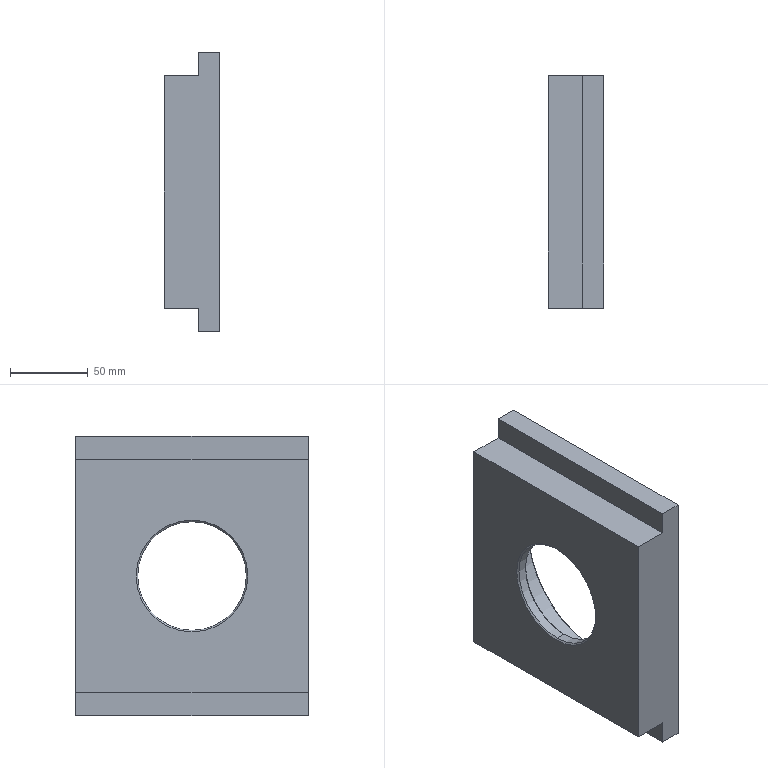Part | SolidWorks | features BaseBody 1 | 1 solid | 34 faces | box 36 x 150 x 180 mm | volume 522217 mm3 | cone 12 | plane 12 | cylinder 10 | commonest cylinder face diameters 30.5 x4 70 x2 110 x2 120 x2
STEP:
#1=CARTESIAN_POINT('',(17.,0.,60.));
#2=VERTEX_POINT('',#1);
#3=CARTESIAN_POINT('',(17.,0.,-60.));
#4=VERTEX_POINT('',#3);
#5=CARTESIAN_POINT('',(17.,0.,0.));
#6=DIRECTION('',(1.,0.,0.));
#7=DIRECTION('',(0.,0.,-1.));
#8=AXIS2_PLACEMENT_3D('',#5,#6,#7);
#9=CIRCLE('',#8,60.);
#10=EDGE_CURVE('',#2,#4,#9,.T.);
#11=ORIENTED_EDGE('',*,*,#10,.F.);
#12=CARTESIAN_POINT('',(18.,0.,61.));
#13=VERTEX_POINT('',#12);
#14=CARTESIAN_POINT('',(17.,0.,60.));
#15=DIRECTION('',(0.7071,0.,0.7071));
#16=VECTOR('',#15,1000.);
#17=LINE('',#14,#16);
#18=EDGE_CURVE('',#2,#13,#17,.T.);
#19=ORIENTED_EDGE('',*,*,#18,.T.);
#20=CARTESIAN_POINT('',(18.,0.,-61.));
#21=VERTEX_POINT('',#20);
#22=CARTESIAN_POINT('',(18.,0.,0.));
#23=DIRECTION('',(-1.,0.,0.));
#24=DIRECTION('',(0.,0.,-1.));
#25=AXIS2_PLACEMENT_3D('',#22,#23,#24);
#26=CIRCLE('',#25,61.);
#27=EDGE_CURVE('',#21,#13,#26,.T.);
#28=ORIENTED_EDGE('',*,*,#27,.F.);
#29=CARTESIAN_POINT('',(17.,0.,-60.));
#30=DIRECTION('',(0.7071,0.,-0.7071));
#31=VECTOR('',#30,1000.);
#32=LINE('',#29,#31);
#33=EDGE_CURVE('',#4,#21,#32,.T.);
#34=ORIENTED_EDGE('',*,*,#33,.F.);
#35=EDGE_LOOP('',(#11,#19,#28,#34));
#36=FACE_OUTER_BOUND('',#35,.T.);
#37=CARTESIAN_POINT('',(17.,0.,0.));
#38=DIRECTION('',(1.,0.,0.));
#39=DIRECTION('',(0.,0.,-1.));
#40=AXIS2_PLACEMENT_3D('',#37,#38,#39);
#41=CONICAL_SURFACE('',#40,60.,0.7854);
#42=ADVANCED_FACE('',(#36),#41,.F.);
#43=CARTESIAN_POINT('',(-11.,0.,35.));
#44=VERTEX_POINT('',#43);
#45=CARTESIAN_POINT('',(-11.,0.,-35.));
#46=VERTEX_POINT('',#45);
#47=CARTESIAN_POINT('',(-11.,0.,0.));
#48=DIRECTION('',(1.,0.,0.));
#49=DIRECTION('',(0.,0.,-1.));
#50=AXIS2_PLACEMENT_3D('',#47,#48,#49);
#51=CIRCLE('',#50,35.);
#52=EDGE_CURVE('',#44,#46,#51,.T.);
#53=ORIENTED_EDGE('',*,*,#52,.F.);
#54=CARTESIAN_POINT('',(-10.,0.,36.));
#55=VERTEX_POINT('',#54);
#56=CARTESIAN_POINT('',(-11.,0.,35.));
#57=DIRECTION('',(0.7071,0.,0.7071));
#58=VECTOR('',#57,1000.);
#59=LINE('',#56,#58);
#60=EDGE_CURVE('',#44,#55,#59,.T.);
#61=ORIENTED_EDGE('',*,*,#60,.T.);
#62=CARTESIAN_POINT('',(-10.,0.,-36.));
#63=VERTEX_POINT('',#62);
#64=CARTESIAN_POINT('',(-10.,0.,0.));
#65=DIRECTION('',(-1.,0.,0.));
#66=DIRECTION('',(0.,0.,-1.));
#67=AXIS2_PLACEMENT_3D('',#64,#65,#66);
#68=CIRCLE('',#67,36.);
#69=EDGE_CURVE('',#63,#55,#68,.T.);
#70=ORIENTED_EDGE('',*,*,#69,.F.);
#71=CARTESIAN_POINT('',(-11.,0.,-35.));
#72=DIRECTION('',(0.7071,0.,-0.7071));
#73=VECTOR('',#72,1000.);
#74=LINE('',#71,#73);
#75=EDGE_CURVE('',#46,#63,#74,.T.);
#76=ORIENTED_EDGE('',*,*,#75,.F.);
#77=EDGE_LOOP('',(#53,#61,#70,#76));
#78=FACE_OUTER_BOUND('',#77,.T.);
#79=CARTESIAN_POINT('',(-11.,0.,0.));
#80=DIRECTION('',(1.,0.,0.));
#81=DIRECTION('',(0.,0.,-1.));
#82=AXIS2_PLACEMENT_3D('',#79,#80,#81);
#83=CONICAL_SURFACE('',#82,35.,0.7854);
#84=ADVANCED_FACE('',(#78),#83,.F.);
#85=CARTESIAN_POINT('',(-17.,0.,-35.));
#86=VERTEX_POINT('',#85);
#87=CARTESIAN_POINT('',(-17.,0.,35.));
#88=VERTEX_POINT('',#87);
#89=CARTESIAN_POINT('',(-17.,0.,0.));
#90=DIRECTION('',(-1.,0.,0.));
#91=DIRECTION('',(0.,0.,-1.));
#92=AXIS2_PLACEMENT_3D('',#89,#90,#91);
#93=CIRCLE('',#92,35.);
#94=EDGE_CURVE('',#86,#88,#93,.T.);
#95=ORIENTED_EDGE('',*,*,#94,.F.);
#96=CARTESIAN_POINT('',(-18.,0.,-36.));
#97=VERTEX_POINT('',#96);
#98=CARTESIAN_POINT('',(-18.,0.,-36.));
#99=DIRECTION('',(-0.7071,0.,-0.7071));
#100=VECTOR('',#99,1000.);
#101=LINE('',#98,#100);
#102=EDGE_CURVE('',#86,#97,#101,.T.);
#103=ORIENTED_EDGE('',*,*,#102,.T.);
#104=CARTESIAN_POINT('',(-18.,0.,36.));
#105=VERTEX_POINT('',#104);
#106=CARTESIAN_POINT('',(-18.,0.,0.));
#107=DIRECTION('',(1.,0.,0.));
#108=DIRECTION('',(0.,0.,-1.));
#109=AXIS2_PLACEMENT_3D('',#106,#107,#108);
#110=CIRCLE('',#109,36.);
#111=EDGE_CURVE('',#105,#97,#110,.T.);
#112=ORIENTED_EDGE('',*,*,#111,.F.);
#113=CARTESIAN_POINT('',(-18.,0.,36.));
#114=DIRECTION('',(-0.7071,0.,0.7071));
#115=VECTOR('',#114,1000.);
#116=LINE('',#113,#115);
#117=EDGE_CURVE('',#88,#105,#116,.T.);
#118=ORIENTED_EDGE('',*,*,#117,.F.);
#119=EDGE_LOOP('',(#95,#103,#112,#118));
#120=FACE_OUTER_BOUND('',#119,.T.);
#121=CARTESIAN_POINT('',(-18.,0.,0.));
#122=DIRECTION('',(-1.,0.,0.));
#123=DIRECTION('',(0.,0.,1.));
#124=AXIS2_PLACEMENT_3D('',#121,#122,#123);
#125=CONICAL_SURFACE('',#124,36.,0.7854);
#126=ADVANCED_FACE('',(#120),#125,.F.);
#127=CARTESIAN_POINT('',(-6.,0.,55.));
#128=VERTEX_POINT('',#127);
#129=CARTESIAN_POINT('',(-6.,0.,-55.));
#130=VERTEX_POINT('',#129);
#131=CARTESIAN_POINT('',(-6.,0.,0.));
#132=DIRECTION('',(1.,0.,0.));
#133=DIRECTION('',(0.,0.,-1.));
#134=AXIS2_PLACEMENT_3D('',#131,#132,#133);
#135=CIRCLE('',#134,55.);
#136=EDGE_CURVE('',#128,#130,#135,.T.);
#137=ORIENTED_EDGE('',*,*,#136,.F.);
#138=CARTESIAN_POINT('',(-5.,0.,56.));
#139=VERTEX_POINT('',#138);
#140=CARTESIAN_POINT('',(-6.,0.,55.));
#141=DIRECTION('',(0.7071,0.,0.7071));
#142=VECTOR('',#141,1000.);
#143=LINE('',#140,#142);
#144=EDGE_CURVE('',#128,#139,#143,.T.);
#145=ORIENTED_EDGE('',*,*,#144,.T.);
#146=CARTESIAN_POINT('',(-5.,0.,-56.));
#147=VERTEX_POINT('',#146);
#148=CARTESIAN_POINT('',(-5.,0.,0.));
#149=DIRECTION('',(-1.,0.,0.));
#150=DIRECTION('',(0.,0.,-1.));
#151=AXIS2_PLACEMENT_3D('',#148,#149,#150);
#152=CIRCLE('',#151,56.);
#153=EDGE_CURVE('',#147,#139,#152,.T.);
#154=ORIENTED_EDGE('',*,*,#153,.F.);
#155=CARTESIAN_POINT('',(-6.,0.,-55.));
#156=DIRECTION('',(0.7071,0.,-0.7071));
#157=VECTOR('',#156,1000.);
#158=LINE('',#155,#157);
#159=EDGE_CURVE('',#130,#147,#158,.T.);
#160=ORIENTED_EDGE('',*,*,#159,.F.);
#161=EDGE_LOOP('',(#137,#145,#154,#160));
#162=FACE_OUTER_BOUND('',#161,.T.);
#163=CARTESIAN_POINT('',(-6.,0.,0.));
#164=DIRECTION('',(1.,0.,0.));
#165=DIRECTION('',(0.,0.,-1.));
#166=AXIS2_PLACEMENT_3D('',#163,#164,#165);
#167=CONICAL_SURFACE('',#166,55.,0.7854);
#168=ADVANCED_FACE('',(#162),#167,.F.);
#169=CARTESIAN_POINT('',(0.,70.,-60.25));
#170=VERTEX_POINT('',#169);
#171=CARTESIAN_POINT('',(0.,70.,-29.75));
#172=VERTEX_POINT('',#171);
#173=CARTESIAN_POINT('',(0.,70.,-45.));
#174=DIRECTION('',(0.,1.,0.));
#175=DIRECTION('',(0.,0.,1.));
#176=AXIS2_PLACEMENT_3D('',#173,#174,#175);
#177=CIRCLE('',#176,15.25);
#178=EDGE_CURVE('',#170,#172,#177,.T.);
#179=ORIENTED_EDGE('',*,*,#178,.F.);
#180=CARTESIAN_POINT('',(0.,75.,-60.25));
#181=VERTEX_POINT('',#180);
#182=CARTESIAN_POINT('',(0.,75.,-60.25));
#183=DIRECTION('',(0.,1.,0.));
#184=VECTOR('',#183,1000.);
#185=LINE('',#182,#184);
#186=EDGE_CURVE('',#170,#181,#185,.T.);
#187=ORIENTED_EDGE('',*,*,#186,.T.);
#188=CARTESIAN_POINT('',(0.,75.,-29.75));
#189=VERTEX_POINT('',#188);
#190=CARTESIAN_POINT('',(0.,75.,-45.));
#191=DIRECTION('',(0.,1.,0.));
#192=DIRECTION('',(0.,0.,1.));
#193=AXIS2_PLACEMENT_3D('',#190,#191,#192);
#194=CIRCLE('',#193,15.25);
#195=EDGE_CURVE('',#181,#189,#194,.T.);
#196=ORIENTED_EDGE('',*,*,#195,.T.);
#197=CARTESIAN_POINT('',(0.,75.,-29.75));
#198=DIRECTION('',(0.,1.,0.));
#199=VECTOR('',#198,1000.);
#200=LINE('',#197,#199);
#201=EDGE_CURVE('',#172,#189,#200,.T.);
#202=ORIENTED_EDGE('',*,*,#201,.F.);
#203=EDGE_LOOP('',(#179,#187,#196,#202));
#204=FACE_OUTER_BOUND('',#203,.T.);
#205=CARTESIAN_POINT('',(0.,75.,-45.));
#206=DIRECTION('',(0.,1.,0.));
#207=DIRECTION('',(0.,0.,1.));
#208=AXIS2_PLACEMENT_3D('',#205,#206,#207);
#209=CYLINDRICAL_SURFACE('',#208,15.25);
#210=ADVANCED_FACE('',(#204),#209,.F.);
#211=CARTESIAN_POINT('',(0.,60.837,-45.));
#212=VERTEX_POINT('',#211);
#213=CARTESIAN_POINT('',(0.,70.,-29.75));
#214=DIRECTION('',(0.,0.515,0.8572));
#215=VECTOR('',#214,1000.);
#216=LINE('',#213,#215);
#217=EDGE_CURVE('',#212,#172,#216,.T.);
#218=ORIENTED_EDGE('',*,*,#217,.F.);
#219=CARTESIAN_POINT('',(0.,70.,-60.25));
#220=DIRECTION('',(0.,0.515,-0.8572));
#221=VECTOR('',#220,1000.);
#222=LINE('',#219,#221);
#223=EDGE_CURVE('',#212,#170,#222,.T.);
#224=ORIENTED_EDGE('',*,*,#223,.T.);
#225=ORIENTED_EDGE('',*,*,#178,.T.);
#226=EDGE_LOOP('',(#218,#224,#225));
#227=FACE_OUTER_BOUND('',#226,.T.);
#228=CARTESIAN_POINT('',(0.,70.,-45.));
#229=DIRECTION('',(0.,1.,0.));
#230=DIRECTION('',(0.,0.,1.));
#231=AXIS2_PLACEMENT_3D('',#228,#229,#230);
#232=CONICAL_SURFACE('',#231,15.25,1.03);
#233=ADVANCED_FACE('',(#227),#232,.F.);
#234=CARTESIAN_POINT('',(0.,70.,29.75));
#235=VERTEX_POINT('',#234);
#236=CARTESIAN_POINT('',(0.,70.,60.25));
#237=VERTEX_POINT('',#236);
#238=CARTESIAN_POINT('',(0.,70.,45.));
#239=DIRECTION('',(0.,1.,0.));
#240=DIRECTION('',(0.,0.,1.));
#241=AXIS2_PLACEMENT_3D('',#238,#239,#240);
#242=CIRCLE('',#241,15.25);
#243=EDGE_CURVE('',#235,#237,#242,.T.);
#244=ORIENTED_EDGE('',*,*,#243,.F.);
#245=CARTESIAN_POINT('',(0.,75.,29.75));
#246=VERTEX_POINT('',#245);
#247=CARTESIAN_POINT('',(0.,75.,29.75));
#248=DIRECTION('',(0.,1.,0.));
#249=VECTOR('',#248,1000.);
#250=LINE('',#247,#249);
#251=EDGE_CURVE('',#235,#246,#250,.T.);
#252=ORIENTED_EDGE('',*,*,#251,.T.);
#253=CARTESIAN_POINT('',(0.,75.,60.25));
#254=VERTEX_POINT('',#253);
#255=CARTESIAN_POINT('',(0.,75.,45.));
#256=DIRECTION('',(0.,1.,0.));
#257=DIRECTION('',(0.,0.,1.));
#258=AXIS2_PLACEMENT_3D('',#255,#256,#257);
#259=CIRCLE('',#258,15.25);
#260=EDGE_CURVE('',#246,#254,#259,.T.);
#261=ORIENTED_EDGE('',*,*,#260,.T.);
#262=CARTESIAN_POINT('',(0.,75.,60.25));
#263=DIRECTION('',(0.,1.,0.));
#264=VECTOR('',#263,1000.);
#265=LINE('',#262,#264);
#266=EDGE_CURVE('',#237,#254,#265,.T.);
#267=ORIENTED_EDGE('',*,*,#266,.F.);
#268=EDGE_LOOP('',(#244,#252,#261,#267));
#269=FACE_OUTER_BOUND('',#268,.T.);
#270=CARTESIAN_POINT('',(0.,75.,45.));
#271=DIRECTION('',(0.,1.,0.));
#272=DIRECTION('',(0.,0.,1.));
#273=AXIS2_PLACEMENT_3D('',#270,#271,#272);
#274=CYLINDRICAL_SURFACE('',#273,15.25);
#275=ADVANCED_FACE('',(#269),#274,.F.);
#276=CARTESIAN_POINT('',(0.,60.837,45.));
#277=VERTEX_POINT('',#276);
#278=CARTESIAN_POINT('',(0.,70.,60.25));
#279=DIRECTION('',(0.,0.515,0.8572));
#280=VECTOR('',#279,1000.);
#281=LINE('',#278,#280);
#282=EDGE_CURVE('',#277,#237,#281,.T.);
#283=ORIENTED_EDGE('',*,*,#282,.F.);
#284=CARTESIAN_POINT('',(0.,70.,29.75));
#285=DIRECTION('',(0.,0.515,-0.8572));
#286=VECTOR('',#285,1000.);
#287=LINE('',#284,#286);
#288=EDGE_CURVE('',#277,#235,#287,.T.);
#289=ORIENTED_EDGE('',*,*,#288,.T.);
#290=ORIENTED_EDGE('',*,*,#243,.T.);
#291=EDGE_LOOP('',(#283,#289,#290));
#292=FACE_OUTER_BOUND('',#291,.T.);
#293=CARTESIAN_POINT('',(0.,70.,45.));
#294=DIRECTION('',(0.,1.,0.));
#295=DIRECTION('',(0.,0.,1.));
#296=AXIS2_PLACEMENT_3D('',#293,#294,#295);
#297=CONICAL_SURFACE('',#296,15.25,1.03);
#298=ADVANCED_FACE('',(#292),#297,.F.);
#299=CARTESIAN_POINT('',(-10.,0.,55.));
#300=VERTEX_POINT('',#299);
#301=CARTESIAN_POINT('',(-10.,0.,-55.));
#302=VERTEX_POINT('',#301);
#303=CARTESIAN_POINT('',(-10.,0.,0.));
#304=DIRECTION('',(1.,0.,0.));
#305=DIRECTION('',(0.,0.,-1.));
#306=AXIS2_PLACEMENT_3D('',#303,#304,#305);
#307=CIRCLE('',#306,55.);
#308=EDGE_CURVE('',#300,#302,#307,.T.);
#309=ORIENTED_EDGE('',*,*,#308,.F.);
#310=CARTESIAN_POINT('',(-10.,0.,55.));
#311=DIRECTION('',(1.,0.,0.));
#312=VECTOR('',#311,1000.);
#313=LINE('',#310,#312);
#314=EDGE_CURVE('',#300,#128,#313,.T.);
#315=ORIENTED_EDGE('',*,*,#314,.T.);
#316=ORIENTED_EDGE('',*,*,#136,.T.);
#317=CARTESIAN_POINT('',(-10.,0.,-55.));
#318=DIRECTION('',(1.,0.,0.));
#319=VECTOR('',#318,1000.);
#320=LINE('',#317,#319);
#321=EDGE_CURVE('',#302,#130,#320,.T.);
#322=ORIENTED_EDGE('',*,*,#321,.F.);
#323=EDGE_LOOP('',(#309,#315,#316,#322));
#324=FACE_OUTER_BOUND('',#323,.T.);
#325=CARTESIAN_POINT('',(-10.,0.,0.));
#326=DIRECTION('',(1.,0.,0.));
#327=DIRECTION('',(0.,0.,-1.));
#328=AXIS2_PLACEMENT_3D('',#325,#326,#327);
#329=CYLINDRICAL_SURFACE('',#328,55.);
#330=ADVANCED_FACE('',(#324),#329,.F.);
#331=CARTESIAN_POINT('',(-5.,0.,60.));
#332=VERTEX_POINT('',#331);
#333=CARTESIAN_POINT('',(-5.,0.,-60.));
#334=VERTEX_POINT('',#333);
#335=CARTESIAN_POINT('',(-5.,0.,0.));
#336=DIRECTION('',(1.,0.,0.));
#337=DIRECTION('',(0.,0.,-1.));
#338=AXIS2_PLACEMENT_3D('',#335,#336,#337);
#339=CIRCLE('',#338,60.);
#340=EDGE_CURVE('',#332,#334,#339,.T.);
#341=ORIENTED_EDGE('',*,*,#340,.F.);
#342=CARTESIAN_POINT('',(-5.,0.,60.));
#343=DIRECTION('',(1.,0.,0.));
#344=VECTOR('',#343,1000.);
#345=LINE('',#342,#344);
#346=EDGE_CURVE('',#332,#2,#345,.T.);
#347=ORIENTED_EDGE('',*,*,#346,.T.);
#348=ORIENTED_EDGE('',*,*,#10,.T.);
#349=CARTESIAN_POINT('',(-5.,0.,-60.));
#350=DIRECTION('',(1.,0.,0.));
#351=VECTOR('',#350,1000.);
#352=LINE('',#349,#351);
#353=EDGE_CURVE('',#334,#4,#352,.T.);
#354=ORIENTED_EDGE('',*,*,#353,.F.);
#355=EDGE_LOOP('',(#341,#347,#348,#354));
#356=FACE_OUTER_BOUND('',#355,.T.);
#357=CARTESIAN_POINT('',(-5.,0.,0.));
#358=DIRECTION('',(1.,0.,0.));
#359=DIRECTION('',(0.,0.,-1.));
#360=AXIS2_PLACEMENT_3D('',#357,#358,#359);
#361=CYLINDRICAL_SURFACE('',#360,60.);
#362=ADVANCED_FACE('',(#356),#361,.F.);
#363=ORIENTED_EDGE('',*,*,#52,.T.);
#364=CARTESIAN_POINT('',(18.,0.,-35.));
#365=DIRECTION('',(-1.,0.,0.));
#366=VECTOR('',#365,1000.);
#367=LINE('',#364,#366);
#368=EDGE_CURVE('',#46,#86,#367,.T.);
#369=ORIENTED_EDGE('',*,*,#368,.T.);
#370=ORIENTED_EDGE('',*,*,#94,.T.);
#371=CARTESIAN_POINT('',(18.,0.,35.));
#372=DIRECTION('',(-1.,0.,0.));
#373=VECTOR('',#372,1000.);
#374=LINE('',#371,#373);
#375=EDGE_CURVE('',#44,#88,#374,.T.);
#376=ORIENTED_EDGE('',*,*,#375,.F.);
#377=EDGE_LOOP('',(#363,#369,#370,#376));
#378=FACE_OUTER_BOUND('',#377,.T.);
#379=CARTESIAN_POINT('',(18.,0.,0.));
#380=DIRECTION('',(-1.,0.,0.));
#381=DIRECTION('',(0.,0.,1.));
#382=AXIS2_PLACEMENT_3D('',#379,#380,#381);
#383=CYLINDRICAL_SURFACE('',#382,35.);
#384=ADVANCED_FACE('',(#378),#383,.F.);
#385=ORIENTED_EDGE('',*,*,#368,.F.);
#386=CARTESIAN_POINT('',(-11.,0.,0.));
#387=DIRECTION('',(1.,0.,0.));
#388=DIRECTION('',(0.,0.,-1.));
#389=AXIS2_PLACEMENT_3D('',#386,#387,#388);
#390=CIRCLE('',#389,35.);
#391=EDGE_CURVE('',#46,#44,#390,.T.);
#392=ORIENTED_EDGE('',*,*,#391,.T.);
#393=ORIENTED_EDGE('',*,*,#375,.T.);
#394=CARTESIAN_POINT('',(-17.,0.,0.));
#395=DIRECTION('',(-1.,0.,0.));
#396=DIRECTION('',(0.,0.,-1.));
#397=AXIS2_PLACEMENT_3D('',#394,#395,#396);
#398=CIRCLE('',#397,35.);
#399=EDGE_CURVE('',#88,#86,#398,.T.);
#400=ORIENTED_EDGE('',*,*,#399,.T.);
#401=EDGE_LOOP('',(#385,#392,#393,#400));
#402=FACE_OUTER_BOUND('',#401,.T.);
#403=CARTESIAN_POINT('',(18.,0.,0.));
#404=DIRECTION('',(-1.,0.,0.));
#405=DIRECTION('',(0.,0.,1.));
#406=AXIS2_PLACEMENT_3D('',#403,#404,#405);
#407=CYLINDRICAL_SURFACE('',#406,35.);
#408=ADVANCED_FACE('',(#402),#407,.F.);
#409=ORIENTED_EDGE('',*,*,#27,.T.);
#410=CARTESIAN_POINT('',(18.,0.,0.));
#411=DIRECTION('',(-1.,0.,0.));
#412=DIRECTION('',(0.,0.,-1.));
#413=AXIS2_PLACEMENT_3D('',#410,#411,#412);
#414=CIRCLE('',#413,61.);
#415=EDGE_CURVE('',#13,#21,#414,.T.);
#416=ORIENTED_EDGE('',*,*,#415,.T.);
#417=EDGE_LOOP('',(#409,#416));
#418=FACE_BOUND('',#417,.T.);
#419=CARTESIAN_POINT('',(18.,-75.,-90.));
#420=VERTEX_POINT('',#419);
#421=CARTESIAN_POINT('',(18.,75.,-90.));
#422=VERTEX_POINT('',#421);
#423=CARTESIAN_POINT('',(18.,75.,-90.));
#424=DIRECTION('',(0.,1.,0.));
#425=VECTOR('',#424,1000.);
#426=LINE('',#423,#425);
#427=EDGE_CURVE('',#420,#422,#426,.T.);
#428=ORIENTED_EDGE('',*,*,#427,.T.);
#429=CARTESIAN_POINT('',(18.,75.,90.));
#430=VERTEX_POINT('',#429);
#431=CARTESIAN_POINT('',(18.,75.,90.));
#432=DIRECTION('',(0.,0.,1.));
#433=VECTOR('',#432,1000.);
#434=LINE('',#431,#433);
#435=EDGE_CURVE('',#422,#430,#434,.T.);
#436=ORIENTED_EDGE('',*,*,#435,.T.);
#437=CARTESIAN_POINT('',(18.,-75.,90.));
#438=VERTEX_POINT('',#437);
#439=CARTESIAN_POINT('',(18.,75.,90.));
#440=DIRECTION('',(0.,-1.,0.));
#441=VECTOR('',#440,1000.);
#442=LINE('',#439,#441);
#443=EDGE_CURVE('',#430,#438,#442,.T.);
#444=ORIENTED_EDGE('',*,*,#443,.T.);
#445=CARTESIAN_POINT('',(18.,-75.,90.));
#446=DIRECTION('',(0.,0.,-1.));
#447=VECTOR('',#446,1000.);
#448=LINE('',#445,#447);
#449=EDGE_CURVE('',#438,#420,#448,.T.);
#450=ORIENTED_EDGE('',*,*,#449,.T.);
#451=EDGE_LOOP('',(#428,#436,#444,#450));
#452=FACE_OUTER_BOUND('',#451,.T.);
#453=CARTESIAN_POINT('',(18.,0.,0.));
#454=DIRECTION('',(1.,0.,0.));
#455=DIRECTION('',(0.,0.,-1.));
#456=AXIS2_PLACEMENT_3D('',#453,#454,#455);
#457=PLANE('',#456);
#458=ADVANCED_FACE('',(#418,#452),#457,.T.);
#459=ORIENTED_EDGE('',*,*,#111,.T.);
#460=CARTESIAN_POINT('',(-18.,0.,0.));
#461=DIRECTION('',(1.,0.,0.));
#462=DIRECTION('',(0.,0.,-1.));
#463=AXIS2_PLACEMENT_3D('',#460,#461,#462);
#464=CIRCLE('',#463,36.);
#465=EDGE_CURVE('',#97,#105,#464,.T.);
#466=ORIENTED_EDGE('',*,*,#465,.T.);
#467=EDGE_LOOP('',(#459,#466));
#468=FACE_BOUND('',#467,.T.);
#469=CARTESIAN_POINT('',(-18.,75.,-75.));
#470=VERTEX_POINT('',#469);
#471=CARTESIAN_POINT('',(-18.,75.,75.));
#472=VERTEX_POINT('',#471);
#473=CARTESIAN_POINT('',(-18.,75.,90.));
#474=DIRECTION('',(0.,0.,1.));
#475=VECTOR('',#474,1000.);
#476=LINE('',#473,#475);
#477=EDGE_CURVE('',#470,#472,#476,.T.);
#478=ORIENTED_EDGE('',*,*,#477,.F.);
#479=CARTESIAN_POINT('',(-18.,-75.,-75.));
#480=VERTEX_POINT('',#479);
#481=CARTESIAN_POINT('',(-18.,-75.,-75.));
#482=DIRECTION('',(0.,1.,0.));
#483=VECTOR('',#482,1000.);
#484=LINE('',#481,#483);
#485=EDGE_CURVE('',#480,#470,#484,.T.);
#486=ORIENTED_EDGE('',*,*,#485,.F.);
#487=CARTESIAN_POINT('',(-18.,-75.,75.));
#488=VERTEX_POINT('',#487);
#489=CARTESIAN_POINT('',(-18.,-75.,90.));
#490=DIRECTION('',(0.,0.,-1.));
#491=VECTOR('',#490,1000.);
#492=LINE('',#489,#491);
#493=EDGE_CURVE('',#488,#480,#492,.T.);
#494=ORIENTED_EDGE('',*,*,#493,.F.);
#495=CARTESIAN_POINT('',(-18.,-75.,75.));
#496=DIRECTION('',(0.,1.,0.));
#497=VECTOR('',#496,1000.);
#498=LINE('',#495,#497);
#499=EDGE_CURVE('',#488,#472,#498,.T.);
#500=ORIENTED_EDGE('',*,*,#499,.T.);
#501=EDGE_LOOP('',(#478,#486,#494,#500));
#502=FACE_OUTER_BOUND('',#501,.T.);
#503=CARTESIAN_POINT('',(-18.,0.,0.));
#504=DIRECTION('',(1.,0.,0.));
#505=DIRECTION('',(0.,0.,-1.));
#506=AXIS2_PLACEMENT_3D('',#503,#504,#505);
#507=PLANE('',#506);
#508=ADVANCED_FACE('',(#468,#502),#507,.F.);
#509=CARTESIAN_POINT('',(4.,-75.,-90.));
#510=VERTEX_POINT('',#509);
#511=CARTESIAN_POINT('',(18.,-75.,-90.));
#512=DIRECTION('',(-1.,0.,0.));
#513=VECTOR('',#512,1000.);
#514=LINE('',#511,#513);
#515=EDGE_CURVE('',#420,#510,#514,.T.);
#516=ORIENTED_EDGE('',*,*,#515,.T.);
#517=CARTESIAN_POINT('',(4.,75.,-90.));
#518=VERTEX_POINT('',#517);
#519=CARTESIAN_POINT('',(4.,-75.,-90.));
#520=DIRECTION('',(0.,1.,0.));
#521=VECTOR('',#520,1000.);
#522=LINE('',#519,#521);
#523=EDGE_CURVE('',#510,#518,#522,.T.);
#524=ORIENTED_EDGE('',*,*,#523,.T.);
#525=CARTESIAN_POINT('',(18.,75.,-90.));
#526=DIRECTION('',(-1.,0.,0.));
#527=VECTOR('',#526,1000.);
#528=LINE('',#525,#527);
#529=EDGE_CURVE('',#422,#518,#528,.T.);
#530=ORIENTED_EDGE('',*,*,#529,.F.);
#531=ORIENTED_EDGE('',*,*,#427,.F.);
#532=EDGE_LOOP('',(#516,#524,#530,#531));
#533=FACE_OUTER_BOUND('',#532,.T.);
#534=CARTESIAN_POINT('',(18.,75.,-90.));
#535=DIRECTION('',(0.,0.,1.));
#536=DIRECTION('',(1.,0.,0.));
#537=AXIS2_PLACEMENT_3D('',#534,#535,#536);
#538=PLANE('',#537);
#539=ADVANCED_FACE('',(#533),#538,.F.);
#540=CARTESIAN_POINT('',(0.,75.,-45.));
#541=DIRECTION('',(0.,1.,0.));
#542=DIRECTION('',(0.,0.,1.));
#543=AXIS2_PLACEMENT_3D('',#540,#541,#542);
#544=CIRCLE('',#543,15.25);
#545=EDGE_CURVE('',#189,#181,#544,.T.);
#546=ORIENTED_EDGE('',*,*,#545,.F.);
#547=ORIENTED_EDGE('',*,*,#195,.F.);
#548=EDGE_LOOP('',(#546,#547));
#549=FACE_BOUND('',#548,.T.);
#550=CARTESIAN_POINT('',(0.,75.,45.));
#551=DIRECTION('',(0.,1.,0.));
#552=DIRECTION('',(0.,0.,1.));
#553=AXIS2_PLACEMENT_3D('',#550,#551,#552);
#554=CIRCLE('',#553,15.25);
#555=EDGE_CURVE('',#254,#246,#554,.T.);
#556=ORIENTED_EDGE('',*,*,#555,.F.);
#557=ORIENTED_EDGE('',*,*,#260,.F.);
#558=EDGE_LOOP('',(#556,#557));
#559=FACE_BOUND('',#558,.T.);
#560=ORIENTED_EDGE('',*,*,#529,.T.);
#561=CARTESIAN_POINT('',(4.,75.,-75.));
#562=VERTEX_POINT('',#561);
#563=CARTESIAN_POINT('',(4.,75.,-90.));
#564=DIRECTION('',(0.,0.,-1.));
#565=VECTOR('',#564,1000.);
#566=LINE('',#563,#565);
#567=EDGE_CURVE('',#562,#518,#566,.T.);
#568=ORIENTED_EDGE('',*,*,#567,.F.);
#569=CARTESIAN_POINT('',(-18.,75.,-75.));
#570=DIRECTION('',(1.,0.,0.));
#571=VECTOR('',#570,1000.);
#572=LINE('',#569,#571);
#573=EDGE_CURVE('',#470,#562,#572,.T.);
#574=ORIENTED_EDGE('',*,*,#573,.F.);
#575=ORIENTED_EDGE('',*,*,#477,.T.);
#576=CARTESIAN_POINT('',(4.,75.,75.));
#577=VERTEX_POINT('',#576);
#578=CARTESIAN_POINT('',(-18.,75.,75.));
#579=DIRECTION('',(-1.,0.,0.));
#580=VECTOR('',#579,1000.);
#581=LINE('',#578,#580);
#582=EDGE_CURVE('',#577,#472,#581,.T.);
#583=ORIENTED_EDGE('',*,*,#582,.F.);
#584=CARTESIAN_POINT('',(4.,75.,90.));
#585=VERTEX_POINT('',#584);
#586=CARTESIAN_POINT('',(4.,75.,90.));
#587=DIRECTION('',(0.,0.,-1.));
#588=VECTOR('',#587,1000.);
#589=LINE('',#586,#588);
#590=EDGE_CURVE('',#585,#577,#589,.T.);
#591=ORIENTED_EDGE('',*,*,#590,.F.);
#592=CARTESIAN_POINT('',(18.,75.,90.));
#593=DIRECTION('',(-1.,0.,0.));
#594=VECTOR('',#593,1000.);
#595=LINE('',#592,#594);
#596=EDGE_CURVE('',#430,#585,#595,.T.);
#597=ORIENTED_EDGE('',*,*,#596,.F.);
#598=ORIENTED_EDGE('',*,*,#435,.F.);
#599=EDGE_LOOP('',(#560,#568,#574,#575,#583,#591,#597,#598));
#600=FACE_OUTER_BOUND('',#599,.T.);
#601=CARTESIAN_POINT('',(18.,75.,90.));
#602=DIRECTION('',(0.,-1.,0.));
#603=DIRECTION('',(0.,0.,-1.));
#604=AXIS2_PLACEMENT_3D('',#601,#602,#603);
#605=PLANE('',#604);
#606=ADVANCED_FACE('',(#549,#559,#600),#605,.F.);
#607=ORIENTED_EDGE('',*,*,#596,.T.);
#608=CARTESIAN_POINT('',(4.,-75.,90.));
#609=VERTEX_POINT('',#608);
#610=CARTESIAN_POINT('',(4.,-75.,90.));
#611=DIRECTION('',(0.,1.,0.));
#612=VECTOR('',#611,1000.);
#613=LINE('',#610,#612);
#614=EDGE_CURVE('',#609,#585,#613,.T.);
#615=ORIENTED_EDGE('',*,*,#614,.F.);
#616=CARTESIAN_POINT('',(18.,-75.,90.));
#617=DIRECTION('',(-1.,0.,0.));
#618=VECTOR('',#617,1000.);
#619=LINE('',#616,#618);
#620=EDGE_CURVE('',#438,#609,#619,.T.);
#621=ORIENTED_EDGE('',*,*,#620,.F.);
#622=ORIENTED_EDGE('',*,*,#443,.F.);
#623=EDGE_LOOP('',(#607,#615,#621,#622));
#624=FACE_OUTER_BOUND('',#623,.T.);
#625=CARTESIAN_POINT('',(18.,75.,90.));
#626=DIRECTION('',(0.,0.,-1.));
#627=DIRECTION('',(-1.,0.,0.));
#628=AXIS2_PLACEMENT_3D('',#625,#626,#627);
#629=PLANE('',#628);
#630=ADVANCED_FACE('',(#624),#629,.F.);
#631=CARTESIAN_POINT('',(4.,-75.,-75.));
#632=VERTEX_POINT('',#631);
#633=CARTESIAN_POINT('',(-18.,-75.,-75.));
#634=DIRECTION('',(1.,0.,0.));
#635=VECTOR('',#634,1000.);
#636=LINE('',#633,#635);
#637=EDGE_CURVE('',#480,#632,#636,.T.);
#638=ORIENTED_EDGE('',*,*,#637,.T.);
#639=CARTESIAN_POINT('',(4.,-75.,-90.));
#640=DIRECTION('',(0.,0.,-1.));
#641=VECTOR('',#640,1000.);
#642=LINE('',#639,#641);
#643=EDGE_CURVE('',#632,#510,#642,.T.);
#644=ORIENTED_EDGE('',*,*,#643,.T.);
#645=ORIENTED_EDGE('',*,*,#515,.F.);
#646=ORIENTED_EDGE('',*,*,#449,.F.);
#647=ORIENTED_EDGE('',*,*,#620,.T.);
#648=CARTESIAN_POINT('',(4.,-75.,75.));
#649=VERTEX_POINT('',#648);
#650=CARTESIAN_POINT('',(4.,-75.,90.));
#651=DIRECTION('',(0.,0.,-1.));
#652=VECTOR('',#651,1000.);
#653=LINE('',#650,#652);
#654=EDGE_CURVE('',#609,#649,#653,.T.);
#655=ORIENTED_EDGE('',*,*,#654,.T.);
#656=CARTESIAN_POINT('',(-18.,-75.,75.));
#657=DIRECTION('',(-1.,0.,0.));
#658=VECTOR('',#657,1000.);
#659=LINE('',#656,#658);
#660=EDGE_CURVE('',#649,#488,#659,.T.);
#661=ORIENTED_EDGE('',*,*,#660,.T.);
#662=ORIENTED_EDGE('',*,*,#493,.T.);
#663=EDGE_LOOP('',(#638,#644,#645,#646,#647,#655,#661,#662));
#664=FACE_OUTER_BOUND('',#663,.T.);
#665=CARTESIAN_POINT('',(18.,-75.,90.));
#666=DIRECTION('',(0.,1.,0.));
#667=DIRECTION('',(0.,0.,1.));
#668=AXIS2_PLACEMENT_3D('',#665,#666,#667);
#669=PLANE('',#668);
#670=ADVANCED_FACE('',(#664),#669,.F.);
#671=ORIENTED_EDGE('',*,*,#346,.F.);
#672=CARTESIAN_POINT('',(-5.,0.,0.));
#673=DIRECTION('',(1.,0.,0.));
#674=DIRECTION('',(0.,0.,-1.));
#675=AXIS2_PLACEMENT_3D('',#672,#673,#674);
#676=CIRCLE('',#675,60.);
#677=EDGE_CURVE('',#334,#332,#676,.T.);
#678=ORIENTED_EDGE('',*,*,#677,.F.);
#679=ORIENTED_EDGE('',*,*,#353,.T.);
#680=CARTESIAN_POINT('',(17.,0.,0.));
#681=DIRECTION('',(1.,0.,0.));
#682=DIRECTION('',(0.,0.,-1.));
#683=AXIS2_PLACEMENT_3D('',#680,#681,#682);
#684=CIRCLE('',#683,60.);
#685=EDGE_CURVE('',#4,#2,#684,.T.);
#686=ORIENTED_EDGE('',*,*,#685,.T.);
#687=EDGE_LOOP('',(#671,#678,#679,#686));
#688=FACE_OUTER_BOUND('',#687,.T.);
#689=CARTESIAN_POINT('',(-5.,0.,0.));
#690=DIRECTION('',(1.,0.,0.));
#691=DIRECTION('',(0.,0.,-1.));
#692=AXIS2_PLACEMENT_3D('',#689,#690,#691);
#693=CYLINDRICAL_SURFACE('',#692,60.);
#694=ADVANCED_FACE('',(#688),#693,.F.);
#695=ORIENTED_EDGE('',*,*,#153,.T.);
#696=CARTESIAN_POINT('',(-5.,0.,0.));
#697=DIRECTION('',(-1.,0.,0.));
#698=DIRECTION('',(0.,0.,-1.));
#699=AXIS2_PLACEMENT_3D('',#696,#697,#698);
#700=CIRCLE('',#699,56.);
#701=EDGE_CURVE('',#139,#147,#700,.T.);
#702=ORIENTED_EDGE('',*,*,#701,.T.);
#703=EDGE_LOOP('',(#695,#702));
#704=FACE_BOUND('',#703,.T.);
#705=ORIENTED_EDGE('',*,*,#677,.T.);
#706=ORIENTED_EDGE('',*,*,#340,.T.);
#707=EDGE_LOOP('',(#705,#706));
#708=FACE_OUTER_BOUND('',#707,.T.);
#709=CARTESIAN_POINT('',(-5.,0.,0.));
#710=DIRECTION('',(1.,0.,0.));
#711=DIRECTION('',(0.,0.,-1.));
#712=AXIS2_PLACEMENT_3D('',#709,#710,#711);
#713=PLANE('',#712);
#714=ADVANCED_FACE('',(#704,#708),#713,.T.);
#715=ORIENTED_EDGE('',*,*,#314,.F.);
#716=CARTESIAN_POINT('',(-10.,0.,0.));
#717=DIRECTION('',(1.,0.,0.));
#718=DIRECTION('',(0.,0.,-1.));
#719=AXIS2_PLACEMENT_3D('',#716,#717,#718);
#720=CIRCLE('',#719,55.);
#721=EDGE_CURVE('',#302,#300,#720,.T.);
#722=ORIENTED_EDGE('',*,*,#721,.F.);
#723=ORIENTED_EDGE('',*,*,#321,.T.);
#724=CARTESIAN_POINT('',(-6.,0.,0.));
#725=DIRECTION('',(1.,0.,0.));
#726=DIRECTION('',(0.,0.,-1.));
#727=AXIS2_PLACEMENT_3D('',#724,#725,#726);
#728=CIRCLE('',#727,55.);
#729=EDGE_CURVE('',#130,#128,#728,.T.);
#730=ORIENTED_EDGE('',*,*,#729,.T.);
#731=EDGE_LOOP('',(#715,#722,#723,#730));
#732=FACE_OUTER_BOUND('',#731,.T.);
#733=CARTESIAN_POINT('',(-10.,0.,0.));
#734=DIRECTION('',(1.,0.,0.));
#735=DIRECTION('',(0.,0.,-1.));
#736=AXIS2_PLACEMENT_3D('',#733,#734,#735);
#737=CYLINDRICAL_SURFACE('',#736,55.);
#738=ADVANCED_FACE('',(#732),#737,.F.);
#739=ORIENTED_EDGE('',*,*,#69,.T.);
#740=CARTESIAN_POINT('',(-10.,0.,0.));
#741=DIRECTION('',(-1.,0.,0.));
#742=DIRECTION('',(0.,0.,-1.));
#743=AXIS2_PLACEMENT_3D('',#740,#741,#742);
#744=CIRCLE('',#743,36.);
#745=EDGE_CURVE('',#55,#63,#744,.T.);
#746=ORIENTED_EDGE('',*,*,#745,.T.);
#747=EDGE_LOOP('',(#739,#746));
#748=FACE_BOUND('',#747,.T.);
#749=ORIENTED_EDGE('',*,*,#721,.T.);
#750=ORIENTED_EDGE('',*,*,#308,.T.);
#751=EDGE_LOOP('',(#749,#750));
#752=FACE_OUTER_BOUND('',#751,.T.);
#753=CARTESIAN_POINT('',(-10.,0.,0.));
#754=DIRECTION('',(1.,0.,0.));
#755=DIRECTION('',(0.,0.,-1.));
#756=AXIS2_PLACEMENT_3D('',#753,#754,#755);
#757=PLANE('',#756);
#758=ADVANCED_FACE('',(#748,#752),#757,.T.);
#759=ORIENTED_EDGE('',*,*,#499,.F.);
#760=ORIENTED_EDGE('',*,*,#660,.F.);
#761=CARTESIAN_POINT('',(4.,-75.,75.));
#762=DIRECTION('',(0.,1.,0.));
#763=VECTOR('',#762,1000.);
#764=LINE('',#761,#763);
#765=EDGE_CURVE('',#649,#577,#764,.T.);
#766=ORIENTED_EDGE('',*,*,#765,.T.);
#767=ORIENTED_EDGE('',*,*,#582,.T.);
#768=EDGE_LOOP('',(#759,#760,#766,#767));
#769=FACE_OUTER_BOUND('',#768,.T.);
#770=CARTESIAN_POINT('',(-18.,-75.,75.));
#771=DIRECTION('',(0.,0.,-1.));
#772=DIRECTION('',(-1.,0.,0.));
#773=AXIS2_PLACEMENT_3D('',#770,#771,#772);
#774=PLANE('',#773);
#775=ADVANCED_FACE('',(#769),#774,.F.);
#776=ORIENTED_EDGE('',*,*,#765,.F.);
#777=ORIENTED_EDGE('',*,*,#654,.F.);
#778=ORIENTED_EDGE('',*,*,#614,.T.);
#779=ORIENTED_EDGE('',*,*,#590,.T.);
#780=EDGE_LOOP('',(#776,#777,#778,#779));
#781=FACE_OUTER_BOUND('',#780,.T.);
#782=CARTESIAN_POINT('',(4.,-75.,90.));
#783=DIRECTION('',(1.,0.,0.));
#784=DIRECTION('',(0.,0.,-1.));
#785=AXIS2_PLACEMENT_3D('',#782,#783,#784);
#786=PLANE('',#785);
#787=ADVANCED_FACE('',(#781),#786,.F.);
#788=ORIENTED_EDGE('',*,*,#523,.F.);
#789=ORIENTED_EDGE('',*,*,#643,.F.);
#790=CARTESIAN_POINT('',(4.,-75.,-75.));
#791=DIRECTION('',(0.,1.,0.));
#792=VECTOR('',#791,1000.);
#793=LINE('',#790,#792);
#794=EDGE_CURVE('',#632,#562,#793,.T.);
#795=ORIENTED_EDGE('',*,*,#794,.T.);
#796=ORIENTED_EDGE('',*,*,#567,.T.);
#797=EDGE_LOOP('',(#788,#789,#795,#796));
#798=FACE_OUTER_BOUND('',#797,.T.);
#799=CARTESIAN_POINT('',(4.,-75.,-90.));
#800=DIRECTION('',(1.,0.,0.));
#801=DIRECTION('',(0.,0.,-1.));
#802=AXIS2_PLACEMENT_3D('',#799,#800,#801);
#803=PLANE('',#802);
#804=ADVANCED_FACE('',(#798),#803,.F.);
#805=ORIENTED_EDGE('',*,*,#794,.F.);
#806=ORIENTED_EDGE('',*,*,#637,.F.);
#807=ORIENTED_EDGE('',*,*,#485,.T.);
#808=ORIENTED_EDGE('',*,*,#573,.T.);
#809=EDGE_LOOP('',(#805,#806,#807,#808));
#810=FACE_OUTER_BOUND('',#809,.T.);
#811=CARTESIAN_POINT('',(-18.,-75.,-75.));
#812=DIRECTION('',(0.,0.,1.));
#813=DIRECTION('',(1.,0.,0.));
#814=AXIS2_PLACEMENT_3D('',#811,#812,#813);
#815=PLANE('',#814);
#816=ADVANCED_FACE('',(#810),#815,.F.);
#817=ORIENTED_EDGE('',*,*,#288,.F.);
#818=ORIENTED_EDGE('',*,*,#282,.T.);
#819=CARTESIAN_POINT('',(0.,70.,45.));
#820=DIRECTION('',(0.,1.,0.));
#821=DIRECTION('',(0.,0.,1.));
#822=AXIS2_PLACEMENT_3D('',#819,#820,#821);
#823=CIRCLE('',#822,15.25);
#824=EDGE_CURVE('',#237,#235,#823,.T.);
#825=ORIENTED_EDGE('',*,*,#824,.T.);
#826=EDGE_LOOP('',(#817,#818,#825));
#827=FACE_OUTER_BOUND('',#826,.T.);
#828=CARTESIAN_POINT('',(0.,70.,45.));
#829=DIRECTION('',(0.,1.,0.));
#830=DIRECTION('',(0.,0.,1.));
#831=AXIS2_PLACEMENT_3D('',#828,#829,#830);
#832=CONICAL_SURFACE('',#831,15.25,1.03);
#833=ADVANCED_FACE('',(#827),#832,.F.);
#834=ORIENTED_EDGE('',*,*,#251,.F.);
#835=ORIENTED_EDGE('',*,*,#824,.F.);
#836=ORIENTED_EDGE('',*,*,#266,.T.);
#837=ORIENTED_EDGE('',*,*,#555,.T.);
#838=EDGE_LOOP('',(#834,#835,#836,#837));
#839=FACE_OUTER_BOUND('',#838,.T.);
#840=CARTESIAN_POINT('',(0.,75.,45.));
#841=DIRECTION('',(0.,1.,0.));
#842=DIRECTION('',(0.,0.,1.));
#843=AXIS2_PLACEMENT_3D('',#840,#841,#842);
#844=CYLINDRICAL_SURFACE('',#843,15.25);
#845=ADVANCED_FACE('',(#839),#844,.F.);
#846=ORIENTED_EDGE('',*,*,#223,.F.);
#847=ORIENTED_EDGE('',*,*,#217,.T.);
#848=CARTESIAN_POINT('',(0.,70.,-45.));
#849=DIRECTION('',(0.,1.,0.));
#850=DIRECTION('',(0.,0.,1.));
#851=AXIS2_PLACEMENT_3D('',#848,#849,#850);
#852=CIRCLE('',#851,15.25);
#853=EDGE_CURVE('',#172,#170,#852,.T.);
#854=ORIENTED_EDGE('',*,*,#853,.T.);
#855=EDGE_LOOP('',(#846,#847,#854));
#856=FACE_OUTER_BOUND('',#855,.T.);
#857=CARTESIAN_POINT('',(0.,70.,-45.));
#858=DIRECTION('',(0.,1.,0.));
#859=DIRECTION('',(0.,0.,1.));
#860=AXIS2_PLACEMENT_3D('',#857,#858,#859);
#861=CONICAL_SURFACE('',#860,15.25,1.03);
#862=ADVANCED_FACE('',(#856),#861,.F.);
#863=ORIENTED_EDGE('',*,*,#186,.F.);
#864=ORIENTED_EDGE('',*,*,#853,.F.);
#865=ORIENTED_EDGE('',*,*,#201,.T.);
#866=ORIENTED_EDGE('',*,*,#545,.T.);
#867=EDGE_LOOP('',(#863,#864,#865,#866));
#868=FACE_OUTER_BOUND('',#867,.T.);
#869=CARTESIAN_POINT('',(0.,75.,-45.));
#870=DIRECTION('',(0.,1.,0.));
#871=DIRECTION('',(0.,0.,1.));
#872=AXIS2_PLACEMENT_3D('',#869,#870,#871);
#873=CYLINDRICAL_SURFACE('',#872,15.25);
#874=ADVANCED_FACE('',(#868),#873,.F.);
#875=ORIENTED_EDGE('',*,*,#144,.F.);
#876=ORIENTED_EDGE('',*,*,#729,.F.);
#877=ORIENTED_EDGE('',*,*,#159,.T.);
#878=ORIENTED_EDGE('',*,*,#701,.F.);
#879=EDGE_LOOP('',(#875,#876,#877,#878));
#880=FACE_OUTER_BOUND('',#879,.T.);
#881=CARTESIAN_POINT('',(-6.,0.,0.));
#882=DIRECTION('',(1.,0.,0.));
#883=DIRECTION('',(0.,0.,-1.));
#884=AXIS2_PLACEMENT_3D('',#881,#882,#883);
#885=CONICAL_SURFACE('',#884,55.,0.7854);
#886=ADVANCED_FACE('',(#880),#885,.F.);
#887=ORIENTED_EDGE('',*,*,#102,.F.);
#888=ORIENTED_EDGE('',*,*,#399,.F.);
#889=ORIENTED_EDGE('',*,*,#117,.T.);
#890=ORIENTED_EDGE('',*,*,#465,.F.);
#891=EDGE_LOOP('',(#887,#888,#889,#890));
#892=FACE_OUTER_BOUND('',#891,.T.);
#893=CARTESIAN_POINT('',(-18.,0.,0.));
#894=DIRECTION('',(-1.,0.,0.));
#895=DIRECTION('',(0.,0.,1.));
#896=AXIS2_PLACEMENT_3D('',#893,#894,#895);
#897=CONICAL_SURFACE('',#896,36.,0.7854);
#898=ADVANCED_FACE('',(#892),#897,.F.);
#899=ORIENTED_EDGE('',*,*,#60,.F.);
#900=ORIENTED_EDGE('',*,*,#391,.F.);
#901=ORIENTED_EDGE('',*,*,#75,.T.);
#902=ORIENTED_EDGE('',*,*,#745,.F.);
#903=EDGE_LOOP('',(#899,#900,#901,#902));
#904=FACE_OUTER_BOUND('',#903,.T.);
#905=CARTESIAN_POINT('',(-11.,0.,0.));
#906=DIRECTION('',(1.,0.,0.));
#907=DIRECTION('',(0.,0.,-1.));
#908=AXIS2_PLACEMENT_3D('',#905,#906,#907);
#909=CONICAL_SURFACE('',#908,35.,0.7854);
#910=ADVANCED_FACE('',(#904),#909,.F.);
#911=ORIENTED_EDGE('',*,*,#18,.F.);
#912=ORIENTED_EDGE('',*,*,#685,.F.);
#913=ORIENTED_EDGE('',*,*,#33,.T.);
#914=ORIENTED_EDGE('',*,*,#415,.F.);
#915=EDGE_LOOP('',(#911,#912,#913,#914));
#916=FACE_OUTER_BOUND('',#915,.T.);
#917=CARTESIAN_POINT('',(17.,0.,0.));
#918=DIRECTION('',(1.,0.,0.));
#919=DIRECTION('',(0.,0.,-1.));
#920=AXIS2_PLACEMENT_3D('',#917,#918,#919);
#921=CONICAL_SURFACE('',#920,60.,0.7854);
#922=ADVANCED_FACE('',(#916),#921,.F.);
#923=CLOSED_SHELL('',(#42,#84,#126,#168,#210,#233,#275,#298,#330,#362,#384,#408,#458,#508,#539,#606,#630,#670,#694,#714,#738,#758,#775,#787,#804,#816,#833,#845,#862,#874,#886,#898,#910,#922));
#924=MANIFOLD_SOLID_BREP('',#923);
#925=CARTESIAN_POINT('',(0.,0.,0.));
#926=DIRECTION('',(0.,0.,1.));
#927=DIRECTION('',(1.,0.,0.));
#928=AXIS2_PLACEMENT_3D('',#925,#926,#927);
#929=(LENGTH_UNIT()NAMED_UNIT(*)SI_UNIT(.MILLI.,.METRE.));
#930=UNCERTAINTY_MEASURE_WITH_UNIT(LENGTH_MEASURE(0.00001),#929,'','');
#931=(NAMED_UNIT(*)PLANE_ANGLE_UNIT()SI_UNIT($,.RADIAN.));
#932=(NAMED_UNIT(*)SI_UNIT($,.STERADIAN.)SOLID_ANGLE_UNIT());
#933=(GEOMETRIC_REPRESENTATION_CONTEXT(3)GLOBAL_UNCERTAINTY_ASSIGNED_CONTEXT((#930))GLOBAL_UNIT_ASSIGNED_CONTEXT((#929,#931,#932))REPRESENTATION_CONTEXT('',''));
#934=ADVANCED_BREP_SHAPE_REPRESENTATION('',(#924,#928),#933);